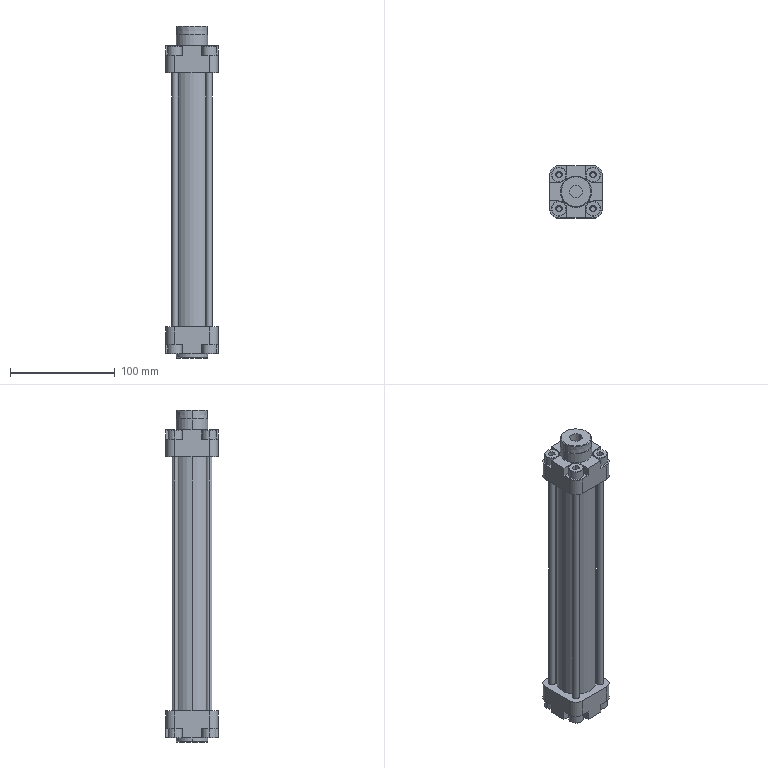Part | STEP file | 1 solid | 306 faces | box 50 x 50 x 317 mm | volume 245584 mm3 | plane 168 | cylinder 86 | cone 36 | torus 16 | commonest cylinder face diameters 4.917 x16 14 x16 6 x12 15.05 x8 17.5 x8 5.9 x4